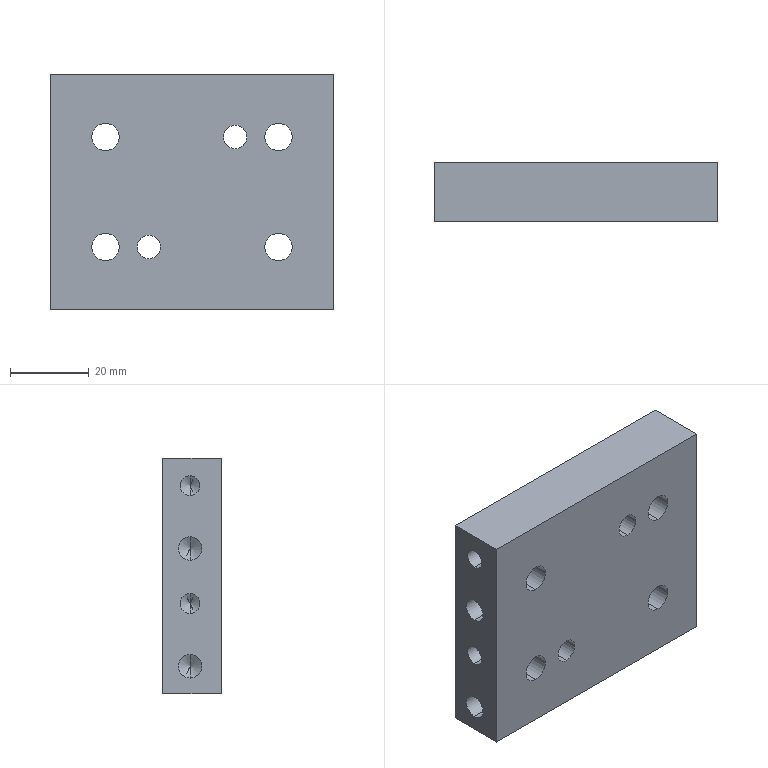Part | STEP file | OP10-155_base plate (F)-L | 1 solid | 50 faces | box 72 x 15 x 60 mm | volume 59226 mm3 | cylinder 28 | cone 16 | plane 6 | commonest cylinder face diameters 6 x12 5 x8 7 x8